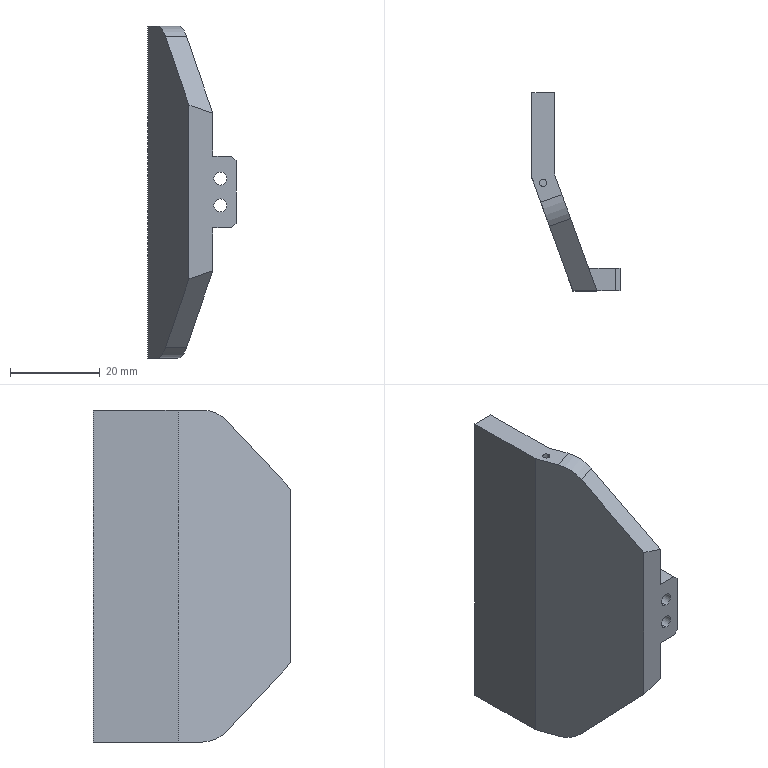NC program | NX | posted with a generic post | part box 19.643 x 44.061 x 74 mm
Whole program, first 1674 of 1956 lines:
N10 G17 G21 G94 G90
(FLOOR_FACING_1_COPY , TOOL : D8开粗)
N12 T02 M6
N14 G54
N16 G17 G0 G90 X-30.186 Y4.36 B0. C0. S5500 M3
N18 G43 Z25.132 H2
N20 Z-1.768
N22 G94 G1 Z-4.768 F800.
N24 X-25.237 Y9.31
N26 G3 X-25.237 Y12.138 R2.
N28 G1 X-33.313 Y20.215
N30 G2 X-35.1 Y24.528 R6.1
N32 G1 Y25.615
N34 X35.1
N36 Y24.528
N38 G2 X33.313 Y20.215 R6.1
N40 G1 X16.77 Y3.672
N42 X12.1
N44 Y11.156
N46 X-12.1
N48 Y3.672
N50 X-16.77
N52 X-25.237 Y12.138
N54 X-20.994 Y16.381
N56 X-24.228 Y19.615
N58 X-28.294 Y21.299
N60 X-24.228 Y19.615
N62 X24.228
N64 X28.294 Y21.299
N66 X24.228 Y19.615
N68 X17.76 Y13.147
N70 X16.306 Y9.144
N72 X17.76 Y13.147
N74 G3 X12.1 Y17.156 R6.
N76 G1 X-12.1
N78 G3 X-17.76 Y13.147 R6.
N80 G1 X-16.306 Y9.144
N82 X-17.76 Y13.147
N84 X-20.994 Y16.381
N86 X-21.701 Y17.088
N88 G3 X-24.53 Y17.088 R2.
N90 G1 X-33.722 Y7.896
N92 Z-1.768
N94 G0 Z25.132
(PLANAR_MILL_4_COPY_1 , TOOL : D8开粗)
N96 X-12.1 Y-6.228
N98 Z-1.768
N100 G1 Z-4.768
N102 Y1.772
N104 Y7.093
N106 G2 X-8. Y11.193 R4.1
N108 G1 X8.
N110 G2 X12.1 Y7.093 R4.1
N112 G1 Y1.772
N114 Y-6.228
N116 Z-1.768
N118 G0 Z25.132
N120 M5
(FLOOR_FACING_1 , TOOL : D8精光)
N122 T03 M6
N124 G54
N126 G17 G0 G90 X-29.964 Y4.28 B0. C0. S5500 M3
N128 G43 Z25.132 H3
N130 Z-1.868
N132 G94 G1 Z-4.868 F800.
N134 X-25.015 Y9.229
N136 G3 X-25.015 Y12.058 R2.
N138 G1 X-33.243 Y20.286
N140 G2 X-35. Y24.528 R6.
N142 G1 Y25.44
N144 X35.
N146 Y24.528
N148 G2 X33.243 Y20.286 R6.
N150 G1 X16.729 Y3.772
N152 X12.
N154 Y11.093
N156 X-12.
N158 Y3.772
N160 X-16.729
N162 X-25.015 Y12.058
N164 X-20.772 Y16.301
N166 X-23.912 Y19.44
N168 X-27.978 Y21.125
N170 X-23.912 Y19.44
N172 X23.912
N174 X27.978 Y21.125
N176 X23.912 Y19.44
N178 X17.632 Y13.161
N180 X16.197 Y9.163
N182 X17.632 Y13.161
N184 G3 X12. Y17.093 R6.
N186 G1 X-12.
N188 G3 X-17.632 Y13.161 R6.
N190 G1 X-16.197 Y9.163
N192 X-17.632 Y13.161
N194 X-20.772 Y16.301
N196 X-21.479 Y17.008
N198 G3 X-24.308 Y17.008 R2.
N200 G1 X-33.5 Y7.815
N202 Z-1.868
N204 G0 Z25.132
(PLANAR_MILL_4 , TOOL : D8精光)
N206 X-12. Y-6.228
N208 Z-1.868
N210 G1 Z-4.868
N212 Y1.772
N214 Y7.093
N216 G2 X-8. Y11.093 R4.
N218 G1 X8.
N220 G2 X12. Y7.093 R4.
N222 G1 Y1.772
N224 Y-6.228
N226 Z-1.868
N228 G0 Z25.132
(PLANAR_MILL_4_COPY , TOOL : D8精光)
N230 X45. Y25.44
N232 Z-1.868
N234 G1 Z-4.868
N236 X37.
N238 X-37.
N240 X-45.
N242 Z-1.868
N244 G0 Z25.132
(PLANAR_MILL_4_COPY_COPY , TOOL : D8精光)
N246 X43. Y26.528
N248 Z-9.868
N250 G1 Z-11.868
N252 G3 X41. Y24.528 R2.
N254 G2 X37.485 Y16.043 R12.
N256 G1 X20.385 Y-1.057
N258 G3 X20.385 Y-3.885 R2.
N260 G1 Z-9.868
N262 G0 Z25.132
N264 X43. Y26.528
N266 Z-9.868
N268 G1 Z-11.868
N270 G3 X41. Y24.528 R2.
N272 G2 X37.485 Y16.043 R12.
N274 G1 X20.385 Y-1.057
N276 G3 X20.385 Y-3.885 R2.
N278 G1 Z-9.868
N280 G0 Z25.132
N282 X-20.385
N284 Z-9.868
N286 G1 Z-11.868
N288 G3 X-20.385 Y-1.057 R2.
N290 G1 X-37.485 Y16.043
N292 G2 X-41. Y24.528 R12.
N294 G3 X-43. Y26.528 R2.
N296 G1 Z-9.868
N298 G0 Z25.132
N300 X-20.385 Y-3.885
N302 Z-9.868
N304 G1 Z-11.868
N306 G3 X-20.385 Y-1.057 R2.
N308 G1 X-37.485 Y16.043
N310 G2 X-41. Y24.528 R12.
N312 G3 X-43. Y26.528 R2.
N314 G1 Z-9.868
N316 G0 Z25.132
N318 M5
(3_AXIS_DEBURRING_1 , TOOL : R1)
N320 T04 M6
N322 G54
N324 G17 G0 G90 X38.707 Y29.103 B0. C0. S4500 M3
N326 G43 Z33.243 H4
N328 Z-4.561
N330 G94 G1 X38.699 Y29.106 Z-4.656 F540.
N332 X38.677 Y29.113 Z-4.748
N334 X38.598 Y29.14 Z-4.926
N336 X38.485 Y29.179 Z-5.087
N338 X38.353 Y29.224 Z-5.226
N340 X38.287 Y29.241 Z-5.274
N342 X38.208 Y29.251 Z-5.304
N344 X38.122 Y29.255 Z-5.32
N346 X38.03 Y29.253 Z-5.322
N348 X37.844 Y29.237 Z-5.293
N350 X37.677 Y29.209 Z-5.231
N352 X37.672 Y29.207 Z-5.228 F600.
N354 Y29.204 Z-5.22
N356 Y29.201 Z-5.212
N358 Y29.198 Z-5.204
N360 Y29.195 Z-5.196
N362 Y28.949
N364 Y28.704
N366 Y28.458
N368 Y28.212
N370 Y27.967
N372 Y27.721
N374 Y27.476
N376 Y27.23
N378 Y26.984
N380 Y26.739
N382 Y26.493
N384 Y26.248
N386 Y26.002
N388 Y25.756
N390 Y25.511
N392 Y25.265
N394 Y25.02
N396 Y24.774
N398 Y24.514
N400 X37.663 Y24.303
N402 X37.654 Y24.11
N404 X37.646 Y23.918
N406 X37.628 Y23.693
N408 X37.599 Y23.466
N410 X37.573 Y23.272
N412 X37.548 Y23.078
N414 X37.503 Y22.854
N416 X37.453 Y22.629
N418 X37.41 Y22.436
N420 X37.363 Y22.243
N422 X37.295 Y22.023
N424 X37.224 Y21.802
N426 X37.165 Y21.613
N428 X37.092 Y21.427
N430 X37.005 Y21.213
N432 X36.915 Y20.999
N434 X36.835 Y20.817
N436 X36.743 Y20.641
N438 X36.637 Y20.435
N440 X36.529 Y20.231
N442 X36.427 Y20.061
N444 X36.321 Y19.894
N446 X36.197 Y19.7
N448 X36.07 Y19.51
N450 X35.951 Y19.354
N452 X35.831 Y19.199
N454 X35.692 Y19.018
N456 X35.545 Y18.847
N458 X35.415 Y18.705
N460 X35.285 Y18.562
N462 X35.142 Y18.407
N464 X34.956 Y18.22
N466 X34.779 Y18.044
N468 X34.603 Y17.868
N470 X34.427 Y17.691
N472 X34.25 Y17.515
N474 X34.074 Y17.339
N476 X33.898 Y17.163
N478 X33.722 Y16.986
N480 X33.545 Y16.81
N482 X33.369 Y16.634
N484 X33.193 Y16.457
N486 X33.016 Y16.281
N488 X32.84 Y16.105
N490 X32.664 Y15.929
N492 X32.488 Y15.752
N494 X32.311 Y15.576
N496 X32.135 Y15.4
N498 X31.959 Y15.223
N500 X31.782 Y15.047
N502 X31.606 Y14.871
N504 X31.43 Y14.695
N506 X31.254 Y14.518
N508 X31.077 Y14.342
N510 X30.901 Y14.166
N512 X30.725 Y13.989
N514 X30.548 Y13.813
N516 X30.372 Y13.637
N518 X30.196 Y13.461
N520 X30.02 Y13.284
N522 X29.843 Y13.108
N524 X29.667 Y12.932
N526 X29.491 Y12.755
N528 X29.314 Y12.579
N530 X29.138 Y12.403
N532 X28.962 Y12.227
N534 X28.786 Y12.05
N536 X28.609 Y11.874
N538 X28.433 Y11.698
N540 X28.257 Y11.521
N542 X28.08 Y11.345
N544 X27.904 Y11.169
N546 X27.728 Y10.993
N548 X27.552 Y10.816
N550 X27.375 Y10.64
N552 X27.199 Y10.464
N554 X27.023 Y10.287
N556 X26.846 Y10.111
N558 X26.67 Y9.935
N560 X26.494 Y9.759
N562 X26.317 Y9.582
N564 X26.141 Y9.406
N566 X25.965 Y9.23
N568 X25.789 Y9.053
N570 X25.612 Y8.877
N572 X25.436 Y8.701
N574 X25.26 Y8.524
N576 X25.083 Y8.348
N578 X24.907 Y8.172
N580 X24.731 Y7.996
N582 X24.555 Y7.819
N584 X24.378 Y7.643
N586 X24.202 Y7.467
N588 X24.026 Y7.29
N590 X23.849 Y7.114
N592 X23.673 Y6.938
N594 X23.497 Y6.762
N596 X23.321 Y6.585
N598 X23.144 Y6.409
N600 X22.968 Y6.233
N602 X22.792 Y6.056
N604 X22.615 Y5.88
N606 X22.439 Y5.704
N608 X22.263 Y5.528
N610 X22.087 Y5.351
N612 X21.91 Y5.175
N614 X21.734 Y4.999
N616 X21.558 Y4.822
N618 X21.381 Y4.646
N620 X21.205 Y4.47
N622 X21.029 Y4.294
N624 X20.853 Y4.117
N626 X20.676 Y3.941
N628 X20.5 Y3.765
N630 X20.324 Y3.588
N632 X20.147 Y3.412
N634 X19.971 Y3.236
N636 X19.795 Y3.06
N638 X19.619 Y2.883
N640 X19.442 Y2.707
N642 X19.266 Y2.531
N644 X19.09 Y2.354
N646 X18.913 Y2.178
N648 X18.737 Y2.002
N650 X18.561 Y1.826
N652 X18.385 Y1.649
N654 X18.208 Y1.473
N656 X18.032 Y1.297
N658 X18.006 Y1.271 Z-5.197
N660 X17.98 Y1.245 Z-5.201
N662 X17.955 Y1.219 Z-5.208
N664 X17.929 Y1.194 Z-5.216
N666 X17.903 Y1.168 Z-5.225
N668 X17.877 Y1.142 Z-5.236
N670 X17.852 Y1.116 Z-5.248
N672 X17.825 Y1.092 Z-5.259
N674 X17.796 Y1.069 Z-5.271
N676 X17.766 Y1.05 Z-5.283
N678 X17.733 Y1.033 Z-5.293
N680 X17.7 Y1.019 Z-5.303
N682 X17.665 Y1.008 Z-5.311
N684 X17.629 Y1. Z-5.317
N686 X17.593 Y0.995 Z-5.321
N688 X17.557 Y0.994 Z-5.323
N690 X17.312
N692 X17.067
N694 X16.822
N696 X16.577
N698 X16.332
N700 X16.087
N702 X15.842
N704 X15.597
N706 X15.352
N708 X15.106
N710 X14.861
N712 X14.616
N714 X14.371
N716 X14.126
N718 X13.881
N720 X13.636
N722 X13.391
N724 X13.146
N726 X12.901
N728 X12.656
N730 X12.411
N732 X12.166
N734 X11.921
N736 X11.676
N738 X11.431
N740 X11.186
N742 X10.941
N744 X10.696
N746 X10.54
N748 X10.443 Y0.982 Z-5.315
N750 X10.345 Y0.949 Z-5.291
N752 X10.27 Y0.897 Z-5.255
N754 X10.248 Y0.865 Z-5.233
N756 X10.24 Y0.83 Z-5.208
N758 Y0.74 Z-5.135
N760 Y0.661 Z-5.046
N762 Y0.605 Z-4.945
N764 Y0.584 Z-4.836
N766 G0 Z0.164
N768 G1 Z0.19
N770 Y0.583 Z0.216
N772 X10.239 Y0.582 Z0.242
N774 X10.238 Y0.581 Z0.269
N776 X10.237 Y0.579 Z0.296
N778 X10.236 Y0.577 Z0.324
N780 X10.234 Y0.574 Z0.352
N782 X10.232 Y0.571 Z0.381
N784 X10.23 Y0.568 Z0.41
N786 X10.228 Y0.564 Z0.44
N788 X10.225 Y0.56 Z0.469
N790 X10.223 Y0.555 Z0.5
N792 X10.22 Y0.551 Z0.531
N794 X10.217 Y0.545 Z0.562
N796 X10.213 Y0.54 Z0.593
N798 X10.21 Y0.534 Z0.625
N800 X10.206 Y0.528 Z0.657
N802 X10.202 Y0.522 Z0.69
N804 X10.198 Y0.515 Z0.723
N806 X10.193 Y0.508 Z0.756
N808 X10.189 Y0.5 Z0.79
N810 X10.184 Y0.492 Z0.823
N812 X10.179 Y0.484 Z0.858
N814 X10.174 Y0.476 Z0.892
N816 X10.168 Y0.468 Z0.926
N818 X10.163 Y0.459 Z0.961
N820 X10.157 Y0.45 Z0.996
N822 X10.151 Y0.44 Z1.032
N824 X10.145 Y0.43 Z1.067
N826 X10.139 Y0.42 Z1.103
N828 X10.133 Y0.41 Z1.139
N830 X10.127 Y0.4 Z1.175
N832 X10.12 Y0.389 Z1.211
N834 X10.113 Y0.378 Z1.248
N836 X10.106 Y0.367 Z1.284
N838 X10.099 Y0.356 Z1.321
N840 X10.092 Y0.344 Z1.358
N842 X10.085 Y0.332 Z1.395
N844 X10.077 Y0.32 Z1.432
N846 X10.07 Y0.308 Z1.469
N848 X10.062 Y0.296 Z1.506
N850 X10.054 Y0.283 Z1.543
N852 X10.046 Y0.27 Z1.581
N854 X10.038 Y0.257 Z1.618
N856 X10.03 Y0.244 Z1.655
N858 X10.022 Y0.231 Z1.693
N860 X10.014 Y0.217 Z1.73
N862 X10.005 Y0.203 Z1.768
N864 X9.997 Y0.19 Z1.805
N866 X9.988 Y0.176 Z1.842
N868 X9.979 Y0.162 Z1.88
N870 X9.971 Y0.147 Z1.917
N872 X9.962 Y0.133 Z1.954
N874 X9.953 Y0.118 Z1.991
N876 X9.944 Y0.104 Z2.028
N878 X9.935 Y0.089 Z2.065
N880 X9.925 Y0.074 Z2.102
N882 X9.916 Y0.059 Z2.139
N884 X9.907 Y0.044 Z2.176
N886 X9.898 Y0.029 Z2.212
N888 X9.888 Y0.014 Z2.249
N890 X9.879 Y-0.001 Z2.285
N892 X9.869 Y-0.017 Z2.321
N894 X9.86 Y-0.032 Z2.357
N896 X9.85 Y-0.048 Z2.392
N898 X9.84 Y-0.063 Z2.428
N900 X9.831 Y-0.079 Z2.463
N902 X9.821 Y-0.095 Z2.498
N904 X9.811 Y-0.111 Z2.533
N906 X9.802 Y-0.126 Z2.567
N908 X9.792 Y-0.142 Z2.602
N910 X9.782 Y-0.158 Z2.636
N912 X9.772 Y-0.174 Z2.669
N914 X9.762 Y-0.19 Z2.703
N916 X9.753 Y-0.206 Z2.736
N918 X9.743 Y-0.222 Z2.768
N920 X9.733 Y-0.237 Z2.801
N922 X9.723 Y-0.253 Z2.833
N924 X9.713 Y-0.269 Z2.865
N926 X9.704 Y-0.285 Z2.896
N928 X9.694 Y-0.301 Z2.927
N930 X9.684 Y-0.317 Z2.958
N932 X9.674 Y-0.332 Z2.988
N934 X9.664 Y-0.348 Z3.018
N936 X9.655 Y-0.364 Z3.047
N938 X9.645 Y-0.38 Z3.076
N940 X9.636 Y-0.395 Z3.105
N942 X9.626 Y-0.411 Z3.133
N944 X9.616 Y-0.426 Z3.16
N946 X9.607 Y-0.442 Z3.187
N948 X9.597 Y-0.457 Z3.214
N950 X9.588 Y-0.472 Z3.24
N952 X9.579 Y-0.487 Z3.266
N954 X9.569 Y-0.502 Z3.291
N956 X9.56 Y-0.517 Z3.316
N958 X9.551 Y-0.532 Z3.34
N960 X9.542 Y-0.547 Z3.363
N962 X9.533 Y-0.561 Z3.386
N964 X9.524 Y-0.576 Z3.408
N966 X9.515 Y-0.59 Z3.43
N968 X9.506 Y-0.605 Z3.451
N970 X9.497 Y-0.619 Z3.472
N972 X9.489 Y-0.633 Z3.492
N974 X9.48 Y-0.646 Z3.511
N976 X9.472 Y-0.66 Z3.53
N978 X9.463 Y-0.674 Z3.547
N980 X9.455 Y-0.687 Z3.565
N982 X9.447 Y-0.7 Z3.581
N984 X9.439 Y-0.713 Z3.597
N986 X9.431 Y-0.726 Z3.613
N988 X9.423 Y-0.739 Z3.627
N990 X9.416 Y-0.751 Z3.641
N992 X9.408 Y-0.763 Z3.654
N994 X9.401 Y-0.775 Z3.666
N996 X9.393 Y-0.787 Z3.678
N998 X9.386 Y-0.799 Z3.689
N1000 X9.379 Y-0.81 Z3.699
N1002 X9.372 Y-0.821 Z3.708
N1004 X9.366 Y-0.832 Z3.716
N1006 X9.359 Y-0.843 Z3.724
N1008 X9.353 Y-0.853 Z3.73
N1010 X9.346 Y-0.863 Z3.736
N1012 X9.34 Y-0.873 Z3.741
N1014 X9.334 Y-0.883 Z3.746
N1016 X9.328 Y-0.893 Z3.749
N1018 X9.323 Y-0.902 Z3.751
N1020 X9.317 Y-0.911 Z3.753
N1022 X9.312 Y-0.919 Z3.754
N1024 X9.307 Y-0.927 Z3.753
N1026 X9.302 Y-0.936 Z3.752
N1028 X9.297 Y-0.943 Z3.75
N1030 X9.292 Y-0.951 Z3.747
N1032 X9.288 Y-0.958 Z3.743
N1034 X9.284 Y-0.965 Z3.738
N1036 X9.28 Y-0.971 Z3.732
N1038 X9.276 Y-0.977 Z3.725
N1040 X9.272 Y-0.983 Z3.717
N1042 X9.269 Y-0.988 Z3.708
N1044 X9.266 Y-0.994 Z3.698
N1046 X9.263 Y-0.998 Z3.687
N1048 X9.26 Y-1.003 Z3.675
N1050 X9.258 Y-1.007 Z3.662
N1052 X9.255 Y-1.011 Z3.647
N1054 X9.253 Y-1.014 Z3.632
N1056 X9.251 Y-1.017 Z3.615
N1058 X9.25 Y-1.02 Z3.598
N1060 X9.248 Y-1.022 Z3.579
N1062 X9.247 Y-1.024 Z3.559
N1064 X9.246 Y-1.025 Z3.538
N1066 Y-1.026 Z3.516
N1068 X9.245 Y-1.027 Z3.493
N1070 Z3.469
N1072 G0 Z-1.532
N1074 G1 X9.239 Y-1.017 Z-1.612 F540.
N1076 X9.222 Y-0.988 Z-1.688
N1078 X9.195 Y-0.943 Z-1.757
N1080 X9.162 Y-0.887 Z-1.819
N1082 X9.081 Y-0.752 Z-1.919
N1084 X8.995 Y-0.609 Z-1.979
N1086 X8.95 Y-0.552 Z-1.987
N1088 X8.892 Y-0.507 Z-1.977
N1090 X8.824 Y-0.473 Z-1.953
N1092 X8.751 Y-0.45 Z-1.918
N1094 X8.602 Y-0.432 Z-1.826
N1096 X8.475 Y-0.452 Z-1.723
N1098 X8.308 Y-0.509 Z-1.566 F600.
N1100 X8.142 Y-0.566 Z-1.41
N1102 X7.975 Y-0.623 Z-1.253
N1104 X7.808 Y-0.68 Z-1.097
N1106 X7.642 Y-0.737 Z-0.94
N1108 X7.475 Y-0.794 Z-0.783
N1110 X7.451 Y-0.801 Z-0.762
N1112 X7.426 Y-0.809 Z-0.742
N1114 X7.4 Y-0.816 Z-0.723
N1116 X7.373 Y-0.822 Z-0.705
N1118 X7.345 Y-0.828 Z-0.688
N1120 X7.317 Y-0.834 Z-0.673
N1122 X7.287 Y-0.839 Z-0.659
N1124 X7.257 Y-0.844 Z-0.647
N1126 X7.226 Y-0.848 Z-0.635
N1128 X7.195 Y-0.851 Z-0.626
N1130 X7.163 Y-0.854 Z-0.617
N1132 X7.131 Y-0.857 Z-0.611
N1134 X7.099 Y-0.859 Z-0.605
N1136 X7.066 Y-0.86 Z-0.602
N1138 X7.033 Y-0.861 Z-0.599
N1140 X7.
N1142 X6.75
N1144 X6.5
N1146 X6.25
N1148 X6.
N1150 X5.75
N1152 X5.5
N1154 X5.25
N1156 X5.
N1158 X4.75
N1160 X4.5
N1162 X4.25
N1164 X4.
N1166 X3.75
N1168 X3.5
N1170 X3.25
N1172 X3.
N1174 X2.75
N1176 X2.5
N1178 X2.25
N1180 X2.
N1182 X1.75
N1184 X1.5
N1186 X1.25
N1188 X1.
N1190 X0.75
N1192 X0.5
N1194 X0.25
N1196 X0.
N1198 X-0.25
N1200 X-0.5
N1202 X-0.75
N1204 X-1.
N1206 X-1.25
N1208 X-1.5
N1210 X-1.75
N1212 X-2.
N1214 X-2.25
N1216 X-2.5
N1218 X-2.75
N1220 X-3.
N1222 X-3.25
N1224 X-3.5
N1226 X-3.75
N1228 X-4.
N1230 X-4.25
N1232 X-4.5
N1234 X-4.75
N1236 X-5.
N1238 X-5.25
N1240 X-5.5
N1242 X-5.75
N1244 X-6.
N1246 X-6.25
N1248 X-6.5
N1250 X-6.75
N1252 X-7.
N1254 X-7.033
N1256 X-7.066 Y-0.86 Z-0.602
N1258 X-7.099 Y-0.859 Z-0.605
N1260 X-7.131 Y-0.857 Z-0.611
N1262 X-7.163 Y-0.854 Z-0.617
N1264 X-7.195 Y-0.851 Z-0.626
N1266 X-7.226 Y-0.848 Z-0.635
N1268 X-7.257 Y-0.844 Z-0.647
N1270 X-7.287 Y-0.839 Z-0.659
N1272 X-7.317 Y-0.834 Z-0.673
N1274 X-7.345 Y-0.828 Z-0.688
N1276 X-7.373 Y-0.822 Z-0.705
N1278 X-7.4 Y-0.816 Z-0.723
N1280 X-7.426 Y-0.809 Z-0.742
N1282 X-7.451 Y-0.801 Z-0.762
N1284 X-7.475 Y-0.794 Z-0.783
N1286 X-7.642 Y-0.737 Z-0.94
N1288 X-7.808 Y-0.68 Z-1.097
N1290 X-7.975 Y-0.623 Z-1.253
N1292 X-8.142 Y-0.566 Z-1.41
N1294 X-8.308 Y-0.509 Z-1.566
N1296 X-8.475 Y-0.452 Z-1.723
N1298 X-8.602 Y-0.432 Z-1.826
N1300 X-8.751 Y-0.45 Z-1.918
N1302 X-8.824 Y-0.473 Z-1.953
N1304 X-8.892 Y-0.507 Z-1.977
N1306 X-8.95 Y-0.552 Z-1.987
N1308 X-8.995 Y-0.609 Z-1.979
N1310 X-9.081 Y-0.752 Z-1.919
N1312 X-9.162 Y-0.887 Z-1.819
N1314 X-9.195 Y-0.943 Z-1.757
N1316 X-9.222 Y-0.988 Z-1.688
N1318 X-9.239 Y-1.017 Z-1.612
N1320 X-9.245 Y-1.027 Z-1.532
N1322 G0 Z3.468
N1324 G1 Z3.493
N1326 X-9.246 Y-1.026 Z3.516
N1328 Y-1.025 Z3.538
N1330 X-9.247 Y-1.024 Z3.559
N1332 X-9.248 Y-1.022 Z3.579
N1334 X-9.25 Y-1.02 Z3.598
N1336 X-9.251 Y-1.017 Z3.615
N1338 X-9.253 Y-1.014 Z3.632
N1340 X-9.255 Y-1.011 Z3.647
N1342 X-9.258 Y-1.007 Z3.662
N1344 X-9.26 Y-1.003 Z3.675
N1346 X-9.263 Y-0.998 Z3.687
N1348 X-9.266 Y-0.994 Z3.698
N1350 X-9.269 Y-0.988 Z3.708
N1352 X-9.272 Y-0.983 Z3.717
N1354 X-9.276 Y-0.977 Z3.725
N1356 X-9.28 Y-0.971 Z3.732
N1358 X-9.284 Y-0.965 Z3.738
N1360 X-9.288 Y-0.958 Z3.743
N1362 X-9.292 Y-0.951 Z3.747
N1364 X-9.297 Y-0.943 Z3.75
N1366 X-9.302 Y-0.936 Z3.752
N1368 X-9.307 Y-0.927 Z3.753
N1370 X-9.312 Y-0.919 Z3.754
N1372 X-9.317 Y-0.911 Z3.753
N1374 X-9.323 Y-0.902 Z3.751
N1376 X-9.328 Y-0.893 Z3.749
N1378 X-9.334 Y-0.883 Z3.746
N1380 X-9.34 Y-0.873 Z3.741
N1382 X-9.346 Y-0.863 Z3.736
N1384 X-9.353 Y-0.853 Z3.73
N1386 X-9.359 Y-0.843 Z3.724
N1388 X-9.366 Y-0.832 Z3.716
N1390 X-9.372 Y-0.821 Z3.708
N1392 X-9.379 Y-0.81 Z3.699
N1394 X-9.386 Y-0.799 Z3.689
N1396 X-9.393 Y-0.787 Z3.678
N1398 X-9.401 Y-0.775 Z3.666
N1400 X-9.408 Y-0.763 Z3.654
N1402 X-9.416 Y-0.751 Z3.641
N1404 X-9.423 Y-0.739 Z3.627
N1406 X-9.431 Y-0.726 Z3.613
N1408 X-9.439 Y-0.713 Z3.597
N1410 X-9.447 Y-0.7 Z3.581
N1412 X-9.455 Y-0.687 Z3.565
N1414 X-9.463 Y-0.674 Z3.547
N1416 X-9.472 Y-0.66 Z3.53
N1418 X-9.48 Y-0.646 Z3.511
N1420 X-9.489 Y-0.633 Z3.492
N1422 X-9.497 Y-0.619 Z3.472
N1424 X-9.506 Y-0.605 Z3.451
N1426 X-9.515 Y-0.59 Z3.43
N1428 X-9.524 Y-0.576 Z3.408
N1430 X-9.533 Y-0.561 Z3.386
N1432 X-9.542 Y-0.547 Z3.363
N1434 X-9.551 Y-0.532 Z3.34
N1436 X-9.56 Y-0.517 Z3.316
N1438 X-9.569 Y-0.502 Z3.291
N1440 X-9.579 Y-0.487 Z3.266
N1442 X-9.588 Y-0.472 Z3.24
N1444 X-9.597 Y-0.457 Z3.214
N1446 X-9.607 Y-0.442 Z3.187
N1448 X-9.616 Y-0.426 Z3.16
N1450 X-9.626 Y-0.411 Z3.133
N1452 X-9.636 Y-0.395 Z3.105
N1454 X-9.645 Y-0.38 Z3.076
N1456 X-9.655 Y-0.364 Z3.047
N1458 X-9.664 Y-0.348 Z3.018
N1460 X-9.674 Y-0.332 Z2.988
N1462 X-9.684 Y-0.317 Z2.958
N1464 X-9.694 Y-0.301 Z2.927
N1466 X-9.704 Y-0.285 Z2.896
N1468 X-9.713 Y-0.269 Z2.865
N1470 X-9.723 Y-0.253 Z2.833
N1472 X-9.733 Y-0.237 Z2.801
N1474 X-9.743 Y-0.222 Z2.768
N1476 X-9.753 Y-0.206 Z2.736
N1478 X-9.762 Y-0.19 Z2.703
N1480 X-9.772 Y-0.174 Z2.669
N1482 X-9.782 Y-0.158 Z2.636
N1484 X-9.792 Y-0.142 Z2.602
N1486 X-9.802 Y-0.126 Z2.567
N1488 X-9.811 Y-0.111 Z2.533
N1490 X-9.821 Y-0.095 Z2.498
N1492 X-9.831 Y-0.079 Z2.463
N1494 X-9.84 Y-0.063 Z2.428
N1496 X-9.85 Y-0.048 Z2.392
N1498 X-9.86 Y-0.032 Z2.357
N1500 X-9.869 Y-0.017 Z2.321
N1502 X-9.879 Y-0.001 Z2.285
N1504 X-9.888 Y0.014 Z2.249
N1506 X-9.898 Y0.029 Z2.212
N1508 X-9.907 Y0.044 Z2.176
N1510 X-9.916 Y0.059 Z2.139
N1512 X-9.925 Y0.074 Z2.102
N1514 X-9.935 Y0.089 Z2.065
N1516 X-9.944 Y0.104 Z2.028
N1518 X-9.953 Y0.118 Z1.991
N1520 X-9.962 Y0.133 Z1.954
N1522 X-9.971 Y0.147 Z1.917
N1524 X-9.979 Y0.162 Z1.88
N1526 X-9.988 Y0.176 Z1.842
N1528 X-9.997 Y0.19 Z1.805
N1530 X-10.005 Y0.203 Z1.768
N1532 X-10.014 Y0.217 Z1.73
N1534 X-10.022 Y0.231 Z1.693
N1536 X-10.03 Y0.244 Z1.655
N1538 X-10.038 Y0.257 Z1.618
N1540 X-10.046 Y0.27 Z1.581
N1542 X-10.054 Y0.283 Z1.543
N1544 X-10.062 Y0.296 Z1.506
N1546 X-10.07 Y0.308 Z1.469
N1548 X-10.077 Y0.32 Z1.432
N1550 X-10.085 Y0.332 Z1.395
N1552 X-10.092 Y0.344 Z1.358
N1554 X-10.099 Y0.356 Z1.321
N1556 X-10.106 Y0.367 Z1.284
N1558 X-10.113 Y0.378 Z1.248
N1560 X-10.12 Y0.389 Z1.211
N1562 X-10.127 Y0.4 Z1.175
N1564 X-10.133 Y0.41 Z1.139
N1566 X-10.139 Y0.42 Z1.103
N1568 X-10.145 Y0.43 Z1.067
N1570 X-10.151 Y0.44 Z1.032
N1572 X-10.157 Y0.45 Z0.996
N1574 X-10.163 Y0.459 Z0.961
N1576 X-10.168 Y0.468 Z0.926
N1578 X-10.174 Y0.476 Z0.892
N1580 X-10.179 Y0.484 Z0.858
N1582 X-10.184 Y0.492 Z0.823
N1584 X-10.189 Y0.5 Z0.79
N1586 X-10.193 Y0.508 Z0.756
N1588 X-10.198 Y0.515 Z0.723
N1590 X-10.202 Y0.522 Z0.69
N1592 X-10.206 Y0.528 Z0.657
N1594 X-10.21 Y0.534 Z0.625
N1596 X-10.213 Y0.54 Z0.593
N1598 X-10.217 Y0.545 Z0.562
N1600 X-10.22 Y0.551 Z0.531
N1602 X-10.223 Y0.555 Z0.5
N1604 X-10.225 Y0.56 Z0.469
N1606 X-10.228 Y0.564 Z0.44
N1608 X-10.23 Y0.568 Z0.41
N1610 X-10.232 Y0.571 Z0.381
N1612 X-10.234 Y0.574 Z0.352
N1614 X-10.236 Y0.577 Z0.324
N1616 X-10.237 Y0.579 Z0.296
N1618 X-10.238 Y0.581 Z0.269
N1620 X-10.239 Y0.582 Z0.242
N1622 X-10.24 Y0.583 Z0.216
N1624 Y0.584 Z0.19
N1626 Z0.164
N1628 G0 Z-4.836
N1630 G1 Y0.605 Z-4.945 F540.
N1632 Y0.661 Z-5.046
N1634 Y0.74 Z-5.135
N1636 Y0.83 Z-5.208
N1638 X-10.248 Y0.865 Z-5.233
N1640 X-10.27 Y0.897 Z-5.255
N1642 X-10.345 Y0.949 Z-5.291
N1644 X-10.443 Y0.982 Z-5.315
N1646 X-10.54 Y0.994 Z-5.323
N1648 X-10.696 F600.
N1650 X-10.941
N1652 X-11.186
N1654 X-11.431
N1656 X-11.676
N1658 X-11.921
N1660 X-12.166
N1662 X-12.411
N1664 X-12.656
N1666 X-12.901
N1668 X-13.146
N1670 X-13.391
N1672 X-13.636
N1674 X-13.881
N1676 X-14.126
N1678 X-14.371
N1680 X-14.616
N1682 X-14.861
N1684 X-15.106
N1686 X-15.352
N1688 X-15.597
N1690 X-15.842
N1692 X-16.087
N1694 X-16.332
N1696 X-16.577
N1698 X-16.822
N1700 X-17.067
N1702 X-17.312
N1704 X-17.557
N1706 X-17.593 Y0.995 Z-5.321
N1708 X-17.629 Y1. Z-5.317
N1710 X-17.665 Y1.008 Z-5.311
N1712 X-17.7 Y1.019 Z-5.303
N1714 X-17.733 Y1.033 Z-5.293
N1716 X-17.766 Y1.05 Z-5.283
N1718 X-17.796 Y1.069 Z-5.271
N1720 X-17.825 Y1.092 Z-5.259
N1722 X-17.852 Y1.116 Z-5.248
N1724 X-17.877 Y1.142 Z-5.236
N1726 X-17.903 Y1.168 Z-5.225
N1728 X-17.929 Y1.194 Z-5.216
N1730 X-17.955 Y1.219 Z-5.208
N1732 X-17.98 Y1.245 Z-5.201
N1734 X-18.006 Y1.271 Z-5.197
N1736 X-18.032 Y1.297 Z-5.196
N1738 X-18.208 Y1.473
N1740 X-18.385 Y1.649
N1742 X-18.561 Y1.826
N1744 X-18.737 Y2.002
N1746 X-18.913 Y2.178
N1748 X-19.09 Y2.354
N1750 X-19.266 Y2.531
N1752 X-19.442 Y2.707
N1754 X-19.619 Y2.883
N1756 X-19.795 Y3.06
N1758 X-19.971 Y3.236
N1760 X-20.147 Y3.412
N1762 X-20.324 Y3.588
N1764 X-20.5 Y3.765
N1766 X-20.676 Y3.941
N1768 X-20.853 Y4.117
N1770 X-21.029 Y4.294
N1772 X-21.205 Y4.47
N1774 X-21.381 Y4.646
N1776 X-21.558 Y4.822
N1778 X-21.734 Y4.999
N1780 X-21.91 Y5.175
N1782 X-22.087 Y5.351
N1784 X-22.263 Y5.528
N1786 X-22.439 Y5.704
N1788 X-22.615 Y5.88
N1790 X-22.792 Y6.056
N1792 X-22.968 Y6.233
N1794 X-23.144 Y6.409
N1796 X-23.321 Y6.585
N1798 X-23.497 Y6.762
N1800 X-23.673 Y6.938
N1802 X-23.849 Y7.114
N1804 X-24.026 Y7.29
N1806 X-24.202 Y7.467
N1808 X-24.378 Y7.643
N1810 X-24.555 Y7.819
N1812 X-24.731 Y7.996
N1814 X-24.907 Y8.172
N1816 X-25.083 Y8.348
N1818 X-25.26 Y8.524
N1820 X-25.436 Y8.701
N1822 X-25.612 Y8.877
N1824 X-25.789 Y9.053
N1826 X-25.965 Y9.23
N1828 X-26.141 Y9.406
N1830 X-26.317 Y9.582
N1832 X-26.494 Y9.759
N1834 X-26.67 Y9.935
N1836 X-26.846 Y10.111
N1838 X-27.023 Y10.287
N1840 X-27.199 Y10.464
N1842 X-27.375 Y10.64
N1844 X-27.552 Y10.816
N1846 X-27.728 Y10.993
N1848 X-27.904 Y11.169
N1850 X-28.08 Y11.345
N1852 X-28.257 Y11.521
N1854 X-28.433 Y11.698
N1856 X-28.609 Y11.874
N1858 X-28.786 Y12.05
N1860 X-28.962 Y12.227
N1862 X-29.138 Y12.403
N1864 X-29.314 Y12.579
N1866 X-29.491 Y12.755
N1868 X-29.667 Y12.932
N1870 X-29.843 Y13.108
N1872 X-30.02 Y13.284
N1874 X-30.196 Y13.461
N1876 X-30.372 Y13.637
N1878 X-30.548 Y13.813
N1880 X-30.725 Y13.989
N1882 X-30.901 Y14.166
N1884 X-31.077 Y14.342
N1886 X-31.254 Y14.518
N1888 X-31.43 Y14.695
N1890 X-31.606 Y14.871
N1892 X-31.782 Y15.047
N1894 X-31.959 Y15.223
N1896 X-32.135 Y15.4
N1898 X-32.311 Y15.576
N1900 X-32.488 Y15.752
N1902 X-32.664 Y15.929
N1904 X-32.84 Y16.105
N1906 X-33.016 Y16.281
N1908 X-33.193 Y16.457
N1910 X-33.369 Y16.634
N1912 X-33.545 Y16.81
N1914 X-33.722 Y16.986
N1916 X-33.898 Y17.163
N1918 X-34.074 Y17.339
N1920 X-34.25 Y17.515
N1922 X-34.427 Y17.691
N1924 X-34.603 Y17.868
N1926 X-34.779 Y18.044
N1928 X-34.956 Y18.22
N1930 X-35.142 Y18.407
N1932 X-35.285 Y18.562
N1934 X-35.415 Y18.705
N1936 X-35.545 Y18.847
N1938 X-35.692 Y19.018
N1940 X-35.831 Y19.199
N1942 X-35.951 Y19.354
N1944 X-36.07 Y19.51
N1946 X-36.197 Y19.7
N1948 X-36.321 Y19.894
N1950 X-36.427 Y20.061
N1952 X-36.529 Y20.231
N1954 X-36.637 Y20.435
N1956 X-36.743 Y20.641
N1958 X-36.835 Y20.817
N1960 X-36.915 Y20.999
N1962 X-37.005 Y21.213
N1964 X-37.092 Y21.427
N1966 X-37.165 Y21.613
N1968 X-37.224 Y21.802
N1970 X-37.295 Y22.023
N1972 X-37.363 Y22.243
N1974 X-37.41 Y22.436
N1976 X-37.453 Y22.629
N1978 X-37.503 Y22.854
N1980 X-37.548 Y23.078
N1982 X-37.573 Y23.272
N1984 X-37.599 Y23.466
N1986 X-37.628 Y23.693
N1988 X-37.646 Y23.918
N1990 X-37.654 Y24.11
N1992 X-37.663 Y24.303
N1994 X-37.672 Y24.514
N1996 Y24.774
N1998 Y25.02
N2000 Y25.265
N2002 Y25.511
N2004 Y25.756
N2006 Y26.002
N2008 Y26.248
N2010 Y26.493
N2012 Y26.739
N2014 Y26.984
N2016 Y27.23
N2018 Y27.476
N2020 Y27.721
N2022 Y27.967
N2024 Y28.212
N2026 Y28.458
N2028 Y28.704
N2030 Y28.949
N2032 Y29.195
N2034 Y29.198 Z-5.204
N2036 Y29.201 Z-5.212
N2038 Y29.204 Z-5.22
N2040 Y29.207 Z-5.228
N2042 X-37.677 Y29.209 Z-5.231
N2044 X-37.844 Y29.237 Z-5.293
N2046 X-38.03 Y29.253 Z-5.322
N2048 X-38.122 Y29.255 Z-5.319
N2050 X-38.208 Y29.251 Z-5.304
N2052 X-38.287 Y29.241 Z-5.274
N2054 X-38.353 Y29.224 Z-5.226
N2056 X-38.485 Y29.179 Z-5.087
N2058 X-38.598 Y29.14 Z-4.926
N2060 X-38.677 Y29.113 Z-4.748
N2062 X-38.699 Y29.106 Z-4.656
N2064 X-38.707 Y29.103 Z-4.561
N2066 G0 Z0.439
N2068 G1 X-38.706 Z0.501
N2070 X-38.702 Z0.562
N2072 X-38.696 Z0.622
N2074 X-38.688 Z0.681
N2076 X-38.677 Z0.739
N2078 X-38.664 Z0.797
N2080 X-38.649 Z0.853
N2082 X-38.631 Y29.102 Z0.909
N2084 X-38.612 Z0.964
N2086 X-38.59 Z1.018
N2088 X-38.566 Z1.072
N2090 X-38.54 Y29.101 Z1.124
N2092 X-38.512 Z1.176
N2094 X-38.482 Z1.227
N2096 X-38.45 Z1.277
N2098 X-38.416 Y29.1 Z1.326
N2100 X-38.38 Z1.374
N2102 X-38.342 Z1.422
N2104 X-38.302 Y29.099 Z1.469
N2106 X-38.261 Z1.515
N2108 X-38.217 Y29.098 Z1.56
N2110 X-38.172 Z1.604
N2112 X-38.125 Y29.097 Z1.648
N2114 X-38.077 Z1.691
N2116 X-38.027 Z1.733
N2118 X-37.975 Y29.096 Z1.774
N2120 X-37.921 Z1.814
N2122 X-37.866 Y29.095 Z1.853
N2124 X-37.809 Y29.094 Z1.892
N2126 X-37.751 Z1.93
N2128 X-37.692 Y29.093 Z1.967
N2130 X-37.631 Z2.003
N2132 X-37.568 Y29.092 Z2.038
N2134 X-37.504 Z2.073
N2136 X-37.439 Y29.091 Z2.106
N2138 X-37.373 Y29.09 Z2.139
N2140 X-37.305 Z2.171
N2142 X-37.236 Y29.089 Z2.203
N2144 X-37.165 Y29.088 Z2.233
N2146 X-37.094 Z2.263
N2148 X-37.021 Y29.087 Z2.292
N2150 X-36.947 Y29.086 Z2.32
N2152 X-36.873 Y29.085 Z2.347
N2154 X-36.797 Z2.373
N2156 X-36.72 Y29.084 Z2.399
N2158 X-36.642 Y29.083 Z2.423
N2160 X-36.563 Y29.082 Z2.447
N2162 X-36.483 Z2.47
N2164 X-36.402 Y29.081 Z2.493
N2166 X-36.321 Y29.08 Z2.514
N2168 X-36.238 Y29.079 Z2.535
N2170 X-36.155 Z2.555
N2172 X-36.071 Y29.078 Z2.574
N2174 X-35.986 Y29.077 Z2.592
N2176 X-35.901 Y29.076 Z2.609
N2178 X-35.814 Y29.075 Z2.626
N2180 X-35.728 Y29.074 Z2.642
N2182 X-35.64 Z2.656
N2184 X-35.552 Y29.073 Z2.671
N2186 X-35.464 Y29.072 Z2.684
N2188 X-35.375 Y29.071 Z2.696
N2190 X-35.285 Y29.07 Z2.708
N2192 X-35.195 Y29.069 Z2.719
N2194 X-35.105 Y29.068 Z2.729
N2196 X-35.014 Z2.738
N2198 X-34.923 Y29.067 Z2.747
N2200 X-34.831 Y29.066 Z2.754
N2202 X-34.739 Y29.065 Z2.761
N2204 X-34.647 Y29.064 Z2.767
N2206 X-34.555 Y29.063 Z2.772
N2208 X-34.463 Y29.062 Z2.776
N2210 X-34.37 Y29.061 Z2.78
N2212 X-34.277 Y29.06 Z2.783
N2214 X-34.185 Z2.784
N2216 X-34.092 Y29.059 Z2.785
N2218 X-33.999 Y29.058 Z2.786
N2220 X-33.906 Y29.057 Z2.785
N2222 X-33.813 Y29.056 Z2.784
N2224 X-33.72 Y29.055 Z2.782
N2226 X-33.627 Y29.054 Z2.779
N2228 X-33.535 Y29.053 Z2.775
N2230 X-33.442 Y29.052 Z2.77
N2232 X-33.35 Z2.765
N2234 X-33.258 Y29.051 Z2.758
N2236 X-33.166 Y29.05 Z2.751
N2238 X-33.075 Y29.049 Z2.743
N2240 X-32.984 Y29.048 Z2.735
N2242 X-32.893 Y29.047 Z2.725
N2244 X-32.803 Y29.046 Z2.715
N2246 X-32.713 Y29.045 Z2.704
N2248 X-32.623 Z2.692
N2250 X-32.534 Y29.044 Z2.679
N2252 X-32.445 Y29.043 Z2.665
N2254 X-32.357 Y29.042 Z2.651
N2256 X-32.27 Y29.041 Z2.636
N2258 X-32.183 Y29.04 Z2.62
N2260 X-32.097 Y29.039 Z2.603
N2262 X-32.012 Z2.585
N2264 X-31.927 Y29.038 Z2.567
N2266 X-31.843 Y29.037 Z2.547
N2268 X-31.76 Y29.036 Z2.527
N2270 X-31.677 Y29.035 Z2.506
N2272 X-31.595 Z2.485
N2274 X-31.515 Y29.034 Z2.462
N2276 X-31.435 Y29.033 Z2.439
N2278 X-31.356 Y29.032 Z2.414
N2280 X-31.278 Z2.389
N2282 X-31.201 Y29.031 Z2.364
N2284 X-31.125 Y29.03 Z2.337
N2286 X-31.05 Y29.029 Z2.31
N2288 X-30.976 Z2.281
N2290 X-30.904 Y29.028 Z2.252
N2292 X-30.832 Y29.027 Z2.222
N2294 X-30.762 Z2.192
N2296 X-30.693 Y29.026 Z2.16
N2298 X-30.625 Y29.025 Z2.128
N2300 X-30.559 Z2.095
N2302 X-30.493 Y29.024 Z2.061
N2304 X-30.43 Y29.023 Z2.026
N2306 X-30.367 Z1.99
N2308 X-30.306 Y29.022 Z1.954
N2310 X-30.246 Z1.917
N2312 X-30.188 Y29.021 Z1.879
N2314 X-30.132 Z1.84
N2316 X-30.077 Y29.02 Z1.8
N2318 X-30.023 Z1.76
N2320 X-29.971 Y29.019 Z1.719
N2322 X-29.921 Z1.677
N2324 X-29.872 Y29.018 Z1.634
N2326 X-29.825 Z1.59
N2328 X-29.78 Y29.017 Z1.546
N2330 X-29.737 Z1.5
N2332 X-29.695 Y29.016 Z1.454
N2334 X-29.656 Z1.407
N2336 X-29.618 Z1.36
N2338 X-29.582 Y29.015 Z1.311
N2340 X-29.548 Z1.262
N2342 X-29.516 Z1.211
N2344 X-29.486 Y29.014 Z1.16
N2346 X-29.458 Z1.109
N2348 X-29.432 Z1.056
N2350 X-29.408 Z1.003
N2352 X-29.386 Y29.013 Z0.948
N2354 X-29.366 Z0.893
N2356 X-29.349 Z0.837
N2358 X-29.334 Z0.781
N2360 X-29.321 Z0.723
N2362 X-29.31 Z0.665
N2364 X-29.302 Z0.606
N2366 X-29.296 Z0.546
N2368 X-29.292 Y29.012 Z0.485
N2370 X-29.291 Z0.424
N2372 G0 Z-4.577
N2374 G1 X-29.299 Y29.015 Z-4.672 F540.
N2376 X-29.321 Y29.023 Z-4.764
N2378 X-29.4 Y29.05 Z-4.942
N2380 X-29.513 Y29.089 Z-5.103
N2382 X-29.644 Y29.133 Z-5.242
N2384 X-29.711 Y29.152 Z-5.29
N2386 X-29.79 Y29.169 Z-5.319
N2388 X-29.876 Y29.182 Z-5.333
N2390 X-29.968 Y29.193
N2392 X-30.154 Y29.206 Z-5.299
N2394 X-30.322 Y29.209 Z-5.231
N2396 X-30.33 Y29.208 Z-5.227 F600.
N2398 X-30.331 Y29.206 Z-5.218
N2400 X-30.333 Y29.204 Z-5.208
N2402 X-30.334 Y29.202 Z-5.198
N2404 X-30.335 Y29.2 Z-5.189
N2406 X-30.344 Y28.956 Z-5.181
N2408 X-30.353 Y28.712 Z-5.172
N2410 X-30.362 Y28.467 Z-5.164
N2412 X-30.371 Y28.223 Z-5.156
N2414 X-30.38 Y27.979 Z-5.148
N2416 X-30.389 Y27.735 Z-5.14
N2418 X-30.359 Y27.613 Z-5.168
N2420 X-30.328 Y27.491 Z-5.196
N2422 Y27.246
N2424 Y27.002
N2426 Y26.758
N2428 Y26.514
N2430 Y26.27
N2432 Y26.026
N2434 Y25.781
N2436 X-30.315 Y25.537
N2438 X-30.318 Y25.446 Z-5.188
N2440 X-30.321 Y25.355 Z-5.18
N2442 X-30.301 Y25.266 Z-5.188
N2444 X-30.281 Y25.176 Z-5.196
N2446 X-30.24 Y24.934
N2448 X-30.188 Y24.693 Z-5.195
N2450 X-30.16 Y24.599 Z-5.196
N2452 X-30.132 Y24.506
N2454 X-30.075 Y24.316
N2456 X-29.998 Y24.133
N2458 X-29.92 Y23.937 Z-5.195
N2460 X-29.809 Y23.73 Z-5.196
N2462 X-29.689 Y23.514
N2464 X-29.639 Y23.438
N2466 X-29.589 Y23.362
N2468 X-29.538 Y23.29
N2470 X-29.488 Y23.218
N2472 X-29.34 Y23.024
N2474 X-29.178 Y22.843
N2476 X-29.038 Y22.687
N2478 X-28.885 Y22.535
N2480 X-28.71 Y22.36
N2482 X-28.534 Y22.184
N2484 X-28.359 Y22.009
N2486 X-28.184 Y21.834
N2488 X-28.008 Y21.658
N2490 X-27.833 Y21.483
N2492 X-27.658 Y21.308
N2494 X-27.482 Y21.132
N2496 X-27.307 Y20.957
N2498 X-27.132 Y20.782
N2500 X-26.956 Y20.606
N2502 X-26.781 Y20.431
N2504 X-26.605 Y20.255
N2506 X-26.43 Y20.08
N2508 X-26.255 Y19.905
N2510 X-26.079 Y19.729
N2512 X-25.904 Y19.554
N2514 X-25.729 Y19.379
N2516 X-25.553 Y19.203
N2518 X-25.378 Y19.028
N2520 X-25.203 Y18.853
N2522 X-25.027 Y18.677
N2524 X-24.852 Y18.502
N2526 X-24.676 Y18.326
N2528 X-24.501 Y18.151
N2530 X-24.326 Y17.976
N2532 X-24.15 Y17.8
N2534 X-23.975 Y17.625
N2536 X-23.8 Y17.45
N2538 X-23.624 Y17.274
N2540 X-23.449 Y17.099
N2542 X-23.273 Y16.923
N2544 X-23.098 Y16.748
N2546 X-22.923 Y16.573
N2548 X-22.747 Y16.397
N2550 X-22.572 Y16.222
N2552 X-22.397 Y16.047
N2554 X-22.221 Y15.871
N2556 X-22.046 Y15.696
N2558 X-21.871 Y15.521
N2560 X-21.695 Y15.345
N2562 X-21.52 Y15.17
N2564 X-21.344 Y14.994
N2566 X-21.169 Y14.819
N2568 X-20.994 Y14.644
N2570 X-20.818 Y14.468
N2572 X-20.643 Y14.293
N2574 X-20.468 Y14.118
N2576 X-20.292 Y13.942
N2578 X-20.117 Y13.767
N2580 X-19.942 Y13.592
N2582 X-19.766 Y13.416
N2584 X-19.591 Y13.241
N2586 X-19.415 Y13.065
N2588 X-19.24 Y12.89
N2590 X-19.065 Y12.715
N2592 X-18.889 Y12.539
N2594 X-18.714 Y12.364
N2596 X-18.539 Y12.189
N2598 X-18.363 Y12.013
N2600 X-18.188 Y11.838
N2602 X-18.013 Y11.663
N2604 X-17.837 Y11.487
N2606 X-17.662 Y11.312
N2608 X-17.486 Y11.136
N2610 X-17.311 Y10.961
N2612 X-17.136 Y10.786
N2614 X-16.96 Y10.61
N2616 X-16.785 Y10.435
N2618 X-16.61 Y10.26
N2620 X-16.434 Y10.084
N2622 X-16.259 Y9.909
N2624 X-16.084 Y9.734
N2626 X-15.908 Y9.558
N2628 X-15.733 Y9.383
N2630 X-15.557 Y9.207
N2632 X-15.406 Y9.054
N2634 X-15.25 Y8.914
N2636 X-15.069 Y8.753
N2638 X-14.875 Y8.604
N2640 X-14.717 Y8.495
N2642 X-14.55 Y8.387
N2644 X-14.363 Y8.284
N2646 X-14.174 Y8.182
N2648 X-13.99 Y8.107
N2650 X-13.796 Y8.024 Z-5.195
N2652 X-13.572 Y7.957 Z-5.196
N2654 X-13.334 Y7.888
N2656 X-13.245 Y7.87
N2658 X-13.156 Y7.852
N2660 X-13.069 Y7.836
N2662 X-12.983 Y7.821
N2664 X-12.741 Y7.788
N2666 X-12.498 Y7.775
N2668 X-12.289 Y7.762 Z-5.195
N2670 X-12.081 Y7.764 Z-5.196
N2672 X-11.841
N2674 X-11.601
N2676 X-11.361
N2678 X-11.121
N2680 X-10.881
N2682 X-10.641
N2684 X-10.401
N2686 X-10.161
N2688 X-9.921
N2690 X-9.681
N2692 X-9.441
N2694 X-9.2
N2696 X-8.96
N2698 X-8.72
N2700 X-8.48 Y7.777 Z-5.183
N2702 X-8.414 Y7.787 Z-5.173
N2704 X-8.349 Y7.809 Z-5.151
N2706 X-8.3 Y7.841 Z-5.119
N2708 X-8.281 Y7.882 Z-5.079
N2710 Y7.98 Z-4.953
N2712 Y8.011 Z-4.88
N2714 Y8.023 Z-4.804
N2716 G0 Z0.196
N2718 G1 Z0.238
N2720 Y8.022 Z0.281
N2722 X-8.282 Y8.021 Z0.324
N2724 X-8.283 Y8.019 Z0.369
N2726 X-8.284 Y8.017 Z0.414
N2728 X-8.285 Y8.014 Z0.46
N2730 X-8.287 Y8.011 Z0.507
N2732 X-8.288 Y8.007 Z0.555
N2734 X-8.29 Y8.003 Z0.604
N2736 X-8.293 Y7.999 Z0.653
N2738 X-8.295 Y7.994 Z0.703
N2740 X-8.298 Y7.988 Z0.754
N2742 X-8.301 Y7.982 Z0.806
N2744 X-8.304 Y7.976 Z0.859
N2746 X-8.307 Y7.969 Z0.912
N2748 X-8.311 Y7.962 Z0.966
N2750 X-8.314 Y7.954 Z1.02
N2752 X-8.318 Y7.946 Z1.075
N2754 X-8.322 Y7.938 Z1.131
N2756 X-8.326 Y7.929 Z1.187
N2758 X-8.331 Y7.92 Z1.244
N2760 X-8.335 Y7.911 Z1.302
N2762 X-8.34 Y7.901 Z1.36
N2764 X-8.345 Y7.891 Z1.418
N2766 X-8.35 Y7.88 Z1.477
N2768 X-8.356 Y7.869 Z1.537
N2770 X-8.361 Y7.858 Z1.597
N2772 X-8.367 Y7.846 Z1.657
N2774 X-8.373 Y7.834 Z1.718
N2776 X-8.379 Y7.822 Z1.779
N2778 X-8.385 Y7.809 Z1.841
N2780 X-8.391 Y7.797 Z1.903
N2782 X-8.397 Y7.783 Z1.965
N2784 X-8.404 Y7.77 Z2.028
N2786 X-8.411 Y7.756 Z2.091
N2788 X-8.417 Y7.742 Z2.154
N2790 X-8.424 Y7.728 Z2.217
N2792 X-8.431 Y7.714 Z2.281
N2794 X-8.439 Y7.699 Z2.345
N2796 X-8.446 Y7.684 Z2.409
N2798 X-8.453 Y7.668 Z2.473
N2800 X-8.461 Y7.653 Z2.538
N2802 X-8.469 Y7.637 Z2.602
N2804 X-8.476 Y7.621 Z2.667
N2806 X-8.484 Y7.605 Z2.732
N2808 X-8.492 Y7.589 Z2.797
N2810 X-8.5 Y7.572 Z2.862
N2812 X-8.509 Y7.555 Z2.927
N2814 X-8.517 Y7.538 Z2.992
N2816 X-8.525 Y7.521 Z3.057
N2818 X-8.534 Y7.504 Z3.122
N2820 X-8.542 Y7.486 Z3.187
N2822 X-8.551 Y7.468 Z3.251
N2824 X-8.559 Y7.451 Z3.316
N2826 X-8.568 Y7.433 Z3.381
N2828 X-8.577 Y7.414 Z3.445
N2830 X-8.586 Y7.396 Z3.51
N2832 X-8.595 Y7.378 Z3.574
N2834 X-8.604 Y7.359 Z3.638
N2836 X-8.613 Y7.341 Z3.702
N2838 X-8.622 Y7.322 Z3.766
N2840 X-8.631 Y7.303 Z3.829
N2842 X-8.64 Y7.284 Z3.892
N2844 X-8.65 Y7.265 Z3.955
N2846 X-8.659 Y7.246 Z4.018
N2848 X-8.668 Y7.227 Z4.08
N2850 X-8.678 Y7.207 Z4.142
N2852 X-8.687 Y7.188 Z4.203
N2854 X-8.697 Y7.169 Z4.265
N2856 X-8.706 Y7.149 Z4.325
N2858 X-8.715 Y7.13 Z4.386
N2860 X-8.725 Y7.11 Z4.446
N2862 X-8.734 Y7.091 Z4.505
N2864 X-8.744 Y7.071 Z4.564
N2866 X-8.753 Y7.052 Z4.622
N2868 X-8.763 Y7.032 Z4.68
N2870 X-8.772 Y7.013 Z4.738
N2872 X-8.782 Y6.993 Z4.795
N2874 X-8.792 Y6.974 Z4.851
N2876 X-8.801 Y6.954 Z4.907
N2878 X-8.81 Y6.935 Z4.962
N2880 X-8.82 Y6.915 Z5.016
N2882 X-8.829 Y6.896 Z5.07
N2884 X-8.839 Y6.876 Z5.123
N2886 X-8.848 Y6.857 Z5.175
N2888 X-8.858 Y6.838 Z5.227
N2890 X-8.867 Y6.819 Z5.278
N2892 X-8.876 Y6.8 Z5.328
N2894 X-8.885 Y6.781 Z5.377
N2896 X-8.895 Y6.762 Z5.426
N2898 X-8.904 Y6.743 Z5.474
N2900 X-8.913 Y6.724 Z5.52
N2902 X-8.922 Y6.705 Z5.566
N2904 X-8.931 Y6.687 Z5.612
N2906 X-8.94 Y6.668 Z5.656
N2908 X-8.949 Y6.65 Z5.699
N2910 X-8.958 Y6.632 Z5.742
N2912 X-8.967 Y6.614 Z5.783
N2914 X-8.975 Y6.596 Z5.823
N2916 X-8.984 Y6.579 Z5.863
N2918 X-8.992 Y6.561 Z5.901
N2920 X-9.001 Y6.544 Z5.939
N2922 X-9.009 Y6.526 Z5.975
N2924 X-9.017 Y6.509 Z6.01
N2926 X-9.026 Y6.493 Z6.044
N2928 X-9.034 Y6.476 Z6.078
N2930 X-9.042 Y6.46 Z6.109
N2932 X-9.05 Y6.443 Z6.14
N2934 X-9.057 Y6.427 Z6.17
N2936 X-9.065 Y6.412 Z6.198
N2938 X-9.073 Y6.396 Z6.225
N2940 X-9.08 Y6.381 Z6.251
N2942 X-9.087 Y6.366 Z6.276
N2944 X-9.095 Y6.351 Z6.299
N2946 X-9.102 Y6.337 Z6.321
N2948 X-9.109 Y6.322 Z6.342
N2950 X-9.115 Y6.308 Z6.361
N2952 X-9.122 Y6.295 Z6.379
N2954 X-9.129 Y6.281 Z6.396
N2956 X-9.135 Y6.268 Z6.411
N2958 X-9.141 Y6.255 Z6.425
N2960 X-9.147 Y6.243 Z6.437
N2962 X-9.153 Y6.23 Z6.448
N2964 X-9.159 Y6.218 Z6.458
N2966 X-9.165 Y6.207 Z6.466
N2968 X-9.17 Y6.196 Z6.472
N2970 X-9.176 Y6.185 Z6.477
N2972 X-9.181 Y6.174 Z6.481
N2974 X-9.186 Y6.164 Z6.482
N2976 X-9.19 Y6.154
N2978 X-9.195 Y6.144 Z6.481
N2980 X-9.2 Y6.135 Z6.478
N2982 X-9.204 Y6.127 Z6.473
N2984 X-9.208 Y6.118 Z6.467
N2986 X-9.212 Y6.11 Z6.459
N2988 X-9.215 Y6.103 Z6.449
N2990 X-9.219 Y6.095 Z6.437
N2992 X-9.222 Y6.089 Z6.424
N2994 X-9.225 Y6.082 Z6.409
N2996 X-9.228 Y6.077 Z6.392
N2998 X-9.231 Y6.071 Z6.373
N3000 X-9.233 Y6.066 Z6.353
N3002 X-9.235 Y6.061 Z6.33
N3004 X-9.237 Y6.057 Z6.306
N3006 X-9.239 Y6.054 Z6.28
N3008 X-9.241 Y6.05 Z6.251
N3010 X-9.242 Y6.048 Z6.221
N3012 X-9.243 Y6.045 Z6.189
N3014 X-9.244 Y6.044 Z6.155
N3016 X-9.245 Y6.042 Z6.119
N3018 Z6.081
N3020 Y6.041 Z6.041
N3022 G0 Z1.041
N3024 G1 X-9.224 Y6.021 Z0.85 F540.
N3026 X-9.169 Y5.966 Z0.668
N3028 X-9.089 Y5.887 Z0.5
N3030 X-8.995 Y5.795 Z0.352
N3032 X-8.95 Y5.756 Z0.309
N3034 X-8.892 Y5.715 Z0.288
N3036 X-8.824 Y5.674 Z0.284
N3038 X-8.751 Y5.633 Z0.296
N3040 X-8.602 Y5.56 Z0.355
N3042 X-8.475 Y5.509 Z0.447
N3044 X-8.308 Y5.452 Z0.603 F600.
N3046 X-8.142 Y5.395 Z0.76
N3048 X-7.975 Y5.338 Z0.916
N3050 X-7.808 Y5.281 Z1.073
N3052 X-7.642 Y5.224 Z1.23
N3054 X-7.475 Y5.167 Z1.386
N3056 X-7.451 Y5.159 Z1.408
N3058 X-7.426 Y5.152 Z1.428
N3060 X-7.4 Y5.145 Z1.447
N3062 X-7.373 Y5.139 Z1.465
N3064 X-7.345 Y5.133 Z1.481
N3066 X-7.317 Y5.127 Z1.497
N3068 X-7.287 Y5.122 Z1.51
N3070 X-7.257 Y5.117 Z1.523
N3072 X-7.226 Y5.113 Z1.534
N3074 X-7.195 Y5.11 Z1.544
N3076 X-7.163 Y5.107 Z1.552
N3078 X-7.131 Y5.104 Z1.559
N3080 X-7.099 Y5.102 Z1.564
N3082 X-7.066 Y5.101 Z1.568
N3084 X-7.033 Y5.1 Z1.57
N3086 X-7. Z1.571
N3088 X-6.75
N3090 X-6.5
N3092 X-6.25
N3094 X-6.
N3096 X-5.75
N3098 X-5.5
N3100 X-5.25
N3102 X-5.
N3104 X-4.75
N3106 X-4.5
N3108 X-4.25
N3110 X-4.
N3112 X-3.75
N3114 X-3.5
N3116 X-3.25
N3118 X-3.
N3120 X-2.75
N3122 X-2.5
N3124 X-2.25
N3126 X-2.
N3128 X-1.75
N3130 X-1.5
N3132 X-1.25
N3134 X-1.
N3136 X-0.75
N3138 X-0.5
N3140 X-0.25
N3142 X0.
N3144 X0.25
N3146 X0.5
N3148 X0.75
N3150 X1.
N3152 X1.25
N3154 X1.5
N3156 X1.75
N3158 X2.
N3160 X2.25
N3162 X2.5
N3164 X2.75
N3166 X3.
N3168 X3.25
N3170 X3.5
N3172 X3.75
N3174 X4.
N3176 X4.25
N3178 X4.5
N3180 X4.75
N3182 X5.
N3184 X5.25
N3186 X5.5
N3188 X5.75
N3190 X6.
N3192 X6.25
N3194 X6.5
N3196 X6.75
N3198 X7.
N3200 X7.033 Z1.57
N3202 X7.066 Y5.101 Z1.568
N3204 X7.099 Y5.102 Z1.564
N3206 X7.131 Y5.104 Z1.559
N3208 X7.163 Y5.107 Z1.552
N3210 X7.195 Y5.11 Z1.544
N3212 X7.226 Y5.113 Z1.534
N3214 X7.257 Y5.117 Z1.523
N3216 X7.287 Y5.122 Z1.51
N3218 X7.317 Y5.127 Z1.497
N3220 X7.345 Y5.133 Z1.481
N3222 X7.373 Y5.139 Z1.465
N3224 X7.4 Y5.145 Z1.447
N3226 X7.426 Y5.152 Z1.428
N3228 X7.451 Y5.159 Z1.408
N3230 X7.475 Y5.167 Z1.386
N3232 X7.642 Y5.224 Z1.23
N3234 X7.808 Y5.281 Z1.073
N3236 X7.975 Y5.338 Z0.916
N3238 X8.142 Y5.395 Z0.76
N3240 X8.308 Y5.452 Z0.603
N3242 X8.475 Y5.509 Z0.447
N3244 X8.602 Y5.56 Z0.355
N3246 X8.751 Y5.633 Z0.296
N3248 X8.824 Y5.674 Z0.284
N3250 X8.892 Y5.715 Z0.288
N3252 X8.95 Y5.756 Z0.309
N3254 X8.995 Y5.795 Z0.352
N3256 X9.089 Y5.887 Z0.5
N3258 X9.169 Y5.966 Z0.668
N3260 X9.224 Y6.021 Z0.85
N3262 X9.245 Y6.041 Z1.041
N3264 G0 Z6.041
N3266 G1 Y6.042 Z6.081
N3268 Z6.119
N3270 X9.244 Y6.044 Z6.155
N3272 X9.243 Y6.045 Z6.189
N3274 X9.242 Y6.048 Z6.221
N3276 X9.241 Y6.05 Z6.251
N3278 X9.239 Y6.054 Z6.28
N3280 X9.237 Y6.057 Z6.306
N3282 X9.235 Y6.061 Z6.33
N3284 X9.233 Y6.066 Z6.353
N3286 X9.231 Y6.071 Z6.373
N3288 X9.228 Y6.077 Z6.392
N3290 X9.225 Y6.082 Z6.409
N3292 X9.222 Y6.089 Z6.424
N3294 X9.219 Y6.095 Z6.437
N3296 X9.215 Y6.103 Z6.449
N3298 X9.212 Y6.11 Z6.459
N3300 X9.208 Y6.118 Z6.467
N3302 X9.204 Y6.127 Z6.473
N3304 X9.2 Y6.135 Z6.478
N3306 X9.195 Y6.144 Z6.481
N3308 X9.19 Y6.154 Z6.482
N3310 X9.186 Y6.164
N3312 X9.181 Y6.174 Z6.481
N3314 X9.176 Y6.185 Z6.477
N3316 X9.17 Y6.196 Z6.472
N3318 X9.165 Y6.207 Z6.466
N3320 X9.159 Y6.218 Z6.458
N3322 X9.153 Y6.23 Z6.448
N3324 X9.147 Y6.243 Z6.437
N3326 X9.141 Y6.255 Z6.425
N3328 X9.135 Y6.268 Z6.411
N3330 X9.129 Y6.281 Z6.396
N3332 X9.122 Y6.295 Z6.379
N3334 X9.115 Y6.308 Z6.361
N3336 X9.109 Y6.322 Z6.342
N3338 X9.102 Y6.337 Z6.321
N3340 X9.095 Y6.351 Z6.299
N3342 X9.087 Y6.366 Z6.276